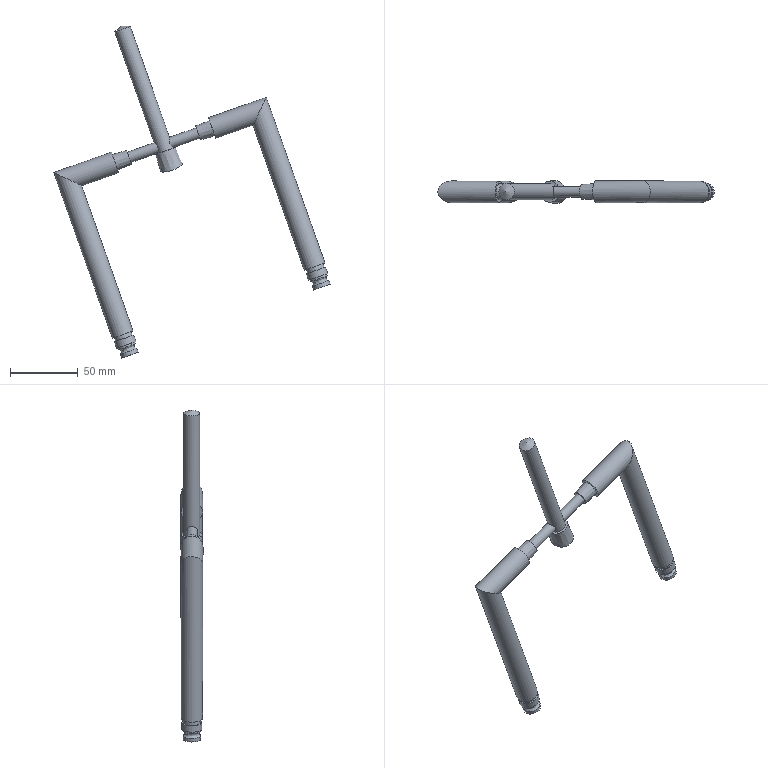Part | STEP file | COOLING-SLIDE1_id166_x_t | 1 solid | 35 faces | box 203.633 x 17.057 x 244.616 mm | volume 86128 mm3 | cylinder 15 | plane 14 | cone 4 | other 2 | commonest cylinder face diameters 13 x6 16 x4 8 x2 15 x2 12 x1
STEP:
#1=CARTESIAN_POINT('',(156.946,0.,-294.272));
#2=VERTEX_POINT('',#1);
#3=CARTESIAN_POINT('',(163.073,0.,-292.102));
#4=DIRECTION('',(-0.3338,0.,0.9426));
#5=DIRECTION('',(-0.9426,0.,-0.3338));
#6=AXIS2_PLACEMENT_3D('',#3,#4,#5);
#7=CIRCLE('',#6,6.5);
#8=EDGE_CURVE('',#2,#2,#7,.T.);
#9=ORIENTED_EDGE('',*,*,#8,.F.);
#10=EDGE_LOOP('',(#9));
#11=FACE_OUTER_BOUND('',#10,.T.);
#12=CARTESIAN_POINT('',(163.073,0.,-292.102));
#13=DIRECTION('',(0.3338,0.,-0.9426));
#14=DIRECTION('',(-0.9426,0.,-0.3338));
#15=AXIS2_PLACEMENT_3D('',#12,#13,#14);
#16=PLANE('',#15);
#17=ADVANCED_FACE('',(#11),#16,.T.);
#18=ORIENTED_EDGE('',*,*,#8,.T.);
#19=EDGE_LOOP('',(#18));
#20=FACE_BOUND('',#19,.T.);
#21=CARTESIAN_POINT('',(168.248,0.,-287.245));
#22=VERTEX_POINT('',#21);
#23=CARTESIAN_POINT('',(162.121,0.,-289.415));
#24=DIRECTION('',(0.3338,0.,-0.9426));
#25=DIRECTION('',(0.9426,0.,0.3338));
#26=AXIS2_PLACEMENT_3D('',#23,#24,#25);
#27=CIRCLE('',#26,6.5);
#28=EDGE_CURVE('',#22,#22,#27,.T.);
#29=ORIENTED_EDGE('',*,*,#28,.T.);
#30=EDGE_LOOP('',(#29));
#31=FACE_BOUND('',#30,.T.);
#32=CARTESIAN_POINT('',(111.159,0.,-145.502));
#33=DIRECTION('',(0.3338,0.,-0.9426));
#34=DIRECTION('',(-0.9426,0.,-0.3338));
#35=AXIS2_PLACEMENT_3D('',#32,#33,#34);
#36=CYLINDRICAL_SURFACE('',#35,6.5);
#37=ADVANCED_FACE('',(#20,#31),#36,.T.);
#38=ORIENTED_EDGE('',*,*,#28,.F.);
#39=EDGE_LOOP('',(#38));
#40=FACE_BOUND('',#39,.T.);
#41=CARTESIAN_POINT('',(154.754,0.,-288.082));
#42=VERTEX_POINT('',#41);
#43=CARTESIAN_POINT('',(160.881,0.,-285.912));
#44=DIRECTION('',(-0.3338,0.,0.9426));
#45=DIRECTION('',(-0.9426,0.,-0.3338));
#46=AXIS2_PLACEMENT_3D('',#43,#44,#45);
#47=CIRCLE('',#46,6.5);
#48=EDGE_CURVE('',#42,#42,#47,.T.);
#49=ORIENTED_EDGE('',*,*,#48,.F.);
#50=EDGE_LOOP('',(#49));
#51=FACE_BOUND('',#50,.T.);
#52=CARTESIAN_POINT('',(168.326,0.,-285.247));
#53=DIRECTION('',(0.,-1.,0.));
#54=DIRECTION('',(0.9426,0.,0.3338));
#55=AXIS2_PLACEMENT_3D('',#52,#53,#54);
#56=CIRCLE('',#55,2.);
#57=CARTESIAN_POINT('',(161.501,0.,-287.664));
#58=DIRECTION('',(0.3338,0.,-0.9426));
#59=AXIS1_PLACEMENT('',#57,#58);
#60=SURFACE_OF_REVOLUTION('',#56,#59);
#61=ADVANCED_FACE('',(#40,#51),#60,.T.);
#62=ORIENTED_EDGE('',*,*,#48,.T.);
#63=EDGE_LOOP('',(#62));
#64=FACE_BOUND('',#63,.T.);
#65=CARTESIAN_POINT('',(154.275,0.,-286.731));
#66=VERTEX_POINT('',#65);
#67=CARTESIAN_POINT('',(160.402,0.,-284.561));
#68=DIRECTION('',(-0.3338,0.,0.9426));
#69=DIRECTION('',(-0.9426,0.,-0.3338));
#70=AXIS2_PLACEMENT_3D('',#67,#68,#69);
#71=CIRCLE('',#70,6.5);
#72=EDGE_CURVE('',#66,#66,#71,.T.);
#73=ORIENTED_EDGE('',*,*,#72,.F.);
#74=EDGE_LOOP('',(#73));
#75=FACE_BOUND('',#74,.T.);
#76=CARTESIAN_POINT('',(111.159,0.,-145.502));
#77=DIRECTION('',(0.3338,0.,-0.9426));
#78=DIRECTION('',(-0.9426,0.,-0.3338));
#79=AXIS2_PLACEMENT_3D('',#76,#77,#78);
#80=CYLINDRICAL_SURFACE('',#79,6.5);
#81=ADVANCED_FACE('',(#64,#75),#80,.T.);
#82=ORIENTED_EDGE('',*,*,#72,.T.);
#83=EDGE_LOOP('',(#82));
#84=FACE_BOUND('',#83,.T.);
#85=CARTESIAN_POINT('',(153.332,0.,-287.065));
#86=VERTEX_POINT('',#85);
#87=CARTESIAN_POINT('',(160.402,0.,-284.561));
#88=DIRECTION('',(-0.3338,0.,0.9426));
#89=DIRECTION('',(-0.9426,0.,-0.3338));
#90=AXIS2_PLACEMENT_3D('',#87,#88,#89);
#91=CIRCLE('',#90,7.5);
#92=EDGE_CURVE('',#86,#86,#91,.T.);
#93=ORIENTED_EDGE('',*,*,#92,.F.);
#94=EDGE_LOOP('',(#93));
#95=FACE_BOUND('',#94,.T.);
#96=CARTESIAN_POINT('',(160.402,0.,-284.561));
#97=DIRECTION('',(0.3338,0.,-0.9426));
#98=DIRECTION('',(-0.9426,0.,-0.3338));
#99=AXIS2_PLACEMENT_3D('',#96,#97,#98);
#100=PLANE('',#99);
#101=ADVANCED_FACE('',(#84,#95),#100,.T.);
#102=CARTESIAN_POINT('',(151.663,0.,-282.351));
#103=VERTEX_POINT('',#102);
#104=CARTESIAN_POINT('',(158.733,0.,-279.848));
#105=DIRECTION('',(0.3338,0.,-0.9426));
#106=DIRECTION('',(-0.9426,0.,-0.3338));
#107=AXIS2_PLACEMENT_3D('',#104,#105,#106);
#108=CIRCLE('',#107,7.5);
#109=EDGE_CURVE('',#103,#103,#108,.T.);
#110=ORIENTED_EDGE('',*,*,#109,.T.);
#111=EDGE_LOOP('',(#110));
#112=FACE_BOUND('',#111,.T.);
#113=ORIENTED_EDGE('',*,*,#92,.T.);
#114=EDGE_LOOP('',(#113));
#115=FACE_BOUND('',#114,.T.);
#116=CARTESIAN_POINT('',(111.159,0.,-145.502));
#117=DIRECTION('',(0.3338,0.,-0.9426));
#118=DIRECTION('',(-0.9426,0.,-0.3338));
#119=AXIS2_PLACEMENT_3D('',#116,#117,#118);
#120=CYLINDRICAL_SURFACE('',#119,7.5);
#121=ADVANCED_FACE('',(#112,#115),#120,.T.);
#122=CARTESIAN_POINT('',(152.606,0.,-282.018));
#123=VERTEX_POINT('',#122);
#124=CARTESIAN_POINT('',(158.733,0.,-279.848));
#125=DIRECTION('',(-0.3338,0.,0.9426));
#126=DIRECTION('',(-0.9426,0.,-0.3338));
#127=AXIS2_PLACEMENT_3D('',#124,#125,#126);
#128=CIRCLE('',#127,6.5);
#129=EDGE_CURVE('',#123,#123,#128,.T.);
#130=ORIENTED_EDGE('',*,*,#129,.F.);
#131=EDGE_LOOP('',(#130));
#132=FACE_BOUND('',#131,.T.);
#133=ORIENTED_EDGE('',*,*,#109,.F.);
#134=EDGE_LOOP('',(#133));
#135=FACE_BOUND('',#134,.T.);
#136=CARTESIAN_POINT('',(158.733,0.,-279.848));
#137=DIRECTION('',(0.3338,0.,-0.9426));
#138=DIRECTION('',(-0.9426,0.,-0.3338));
#139=AXIS2_PLACEMENT_3D('',#136,#137,#138);
#140=PLANE('',#139);
#141=ADVANCED_FACE('',(#132,#135),#140,.F.);
#142=ORIENTED_EDGE('',*,*,#129,.T.);
#143=EDGE_LOOP('',(#142));
#144=FACE_BOUND('',#143,.T.);
#145=CARTESIAN_POINT('',(151.605,0.,-279.19));
#146=VERTEX_POINT('',#145);
#147=CARTESIAN_POINT('',(157.732,0.,-277.02));
#148=DIRECTION('',(-0.3338,0.,0.9426));
#149=DIRECTION('',(-0.9426,0.,-0.3338));
#150=AXIS2_PLACEMENT_3D('',#147,#148,#149);
#151=CIRCLE('',#150,6.5);
#152=EDGE_CURVE('',#146,#146,#151,.T.);
#153=ORIENTED_EDGE('',*,*,#152,.F.);
#154=EDGE_LOOP('',(#153));
#155=FACE_BOUND('',#154,.T.);
#156=CARTESIAN_POINT('',(111.159,0.,-145.502));
#157=DIRECTION('',(0.3338,0.,-0.9426));
#158=DIRECTION('',(-0.9426,0.,-0.3338));
#159=AXIS2_PLACEMENT_3D('',#156,#157,#158);
#160=CYLINDRICAL_SURFACE('',#159,6.5);
#161=ADVANCED_FACE('',(#144,#155),#160,.T.);
#162=ORIENTED_EDGE('',*,*,#152,.T.);
#163=EDGE_LOOP('',(#162));
#164=FACE_BOUND('',#163,.T.);
#165=CARTESIAN_POINT('',(150.191,0.,-279.69));
#166=VERTEX_POINT('',#165);
#167=CARTESIAN_POINT('',(157.732,0.,-277.02));
#168=DIRECTION('',(-0.3338,0.,0.9426));
#169=DIRECTION('',(-0.9426,0.,-0.3338));
#170=AXIS2_PLACEMENT_3D('',#167,#168,#169);
#171=CIRCLE('',#170,8.);
#172=EDGE_CURVE('',#166,#166,#171,.T.);
#173=ORIENTED_EDGE('',*,*,#172,.F.);
#174=EDGE_LOOP('',(#173));
#175=FACE_BOUND('',#174,.T.);
#176=CARTESIAN_POINT('',(157.732,0.,-277.02));
#177=DIRECTION('',(0.3338,0.,-0.9426));
#178=DIRECTION('',(-0.9426,0.,-0.3338));
#179=AXIS2_PLACEMENT_3D('',#176,#177,#178);
#180=PLANE('',#179);
#181=ADVANCED_FACE('',(#164,#175),#180,.T.);
#182=ORIENTED_EDGE('',*,*,#172,.T.);
#183=EDGE_LOOP('',(#182));
#184=FACE_BOUND('',#183,.T.);
#185=CARTESIAN_POINT('',(112.304,0.,-172.701));
#186=VERTEX_POINT('',#185);
#187=CARTESIAN_POINT('',(117.174,0.,-162.489));
#188=DIRECTION('',(-0.9026,0.,0.4305));
#189=DIRECTION('',(-0.4305,0.,-0.9026));
#190=AXIS2_PLACEMENT_3D('',#187,#188,#189);
#191=ELLIPSE('',#190,11.314,8.);
#192=EDGE_CURVE('',#186,#186,#191,.T.);
#193=ORIENTED_EDGE('',*,*,#192,.F.);
#194=EDGE_LOOP('',(#193));
#195=FACE_BOUND('',#194,.T.);
#196=CARTESIAN_POINT('',(111.159,0.,-145.502));
#197=DIRECTION('',(0.3338,0.,-0.9426));
#198=DIRECTION('',(-0.9426,0.,-0.3338));
#199=AXIS2_PLACEMENT_3D('',#196,#197,#198);
#200=CYLINDRICAL_SURFACE('',#199,8.);
#201=ADVANCED_FACE('',(#184,#195),#200,.T.);
#202=CARTESIAN_POINT('',(79.626,0.,-167.299));
#203=VERTEX_POINT('',#202);
#204=CARTESIAN_POINT('',(82.297,0.,-174.84));
#205=DIRECTION('',(-0.9426,0.,-0.3338));
#206=DIRECTION('',(-0.3338,0.,0.9426));
#207=AXIS2_PLACEMENT_3D('',#204,#205,#206);
#208=CIRCLE('',#207,8.);
#209=EDGE_CURVE('',#203,#203,#208,.T.);
#210=ORIENTED_EDGE('',*,*,#209,.F.);
#211=EDGE_LOOP('',(#210));
#212=FACE_BOUND('',#211,.T.);
#213=ORIENTED_EDGE('',*,*,#192,.T.);
#214=EDGE_LOOP('',(#213));
#215=FACE_BOUND('',#214,.T.);
#216=CARTESIAN_POINT('',(135.149,0.,-156.124));
#217=DIRECTION('',(-0.9426,0.,-0.3338));
#218=DIRECTION('',(-0.3338,0.,0.9426));
#219=AXIS2_PLACEMENT_3D('',#216,#217,#218);
#220=CYLINDRICAL_SURFACE('',#219,8.);
#221=ADVANCED_FACE('',(#212,#215),#220,.T.);
#222=CARTESIAN_POINT('',(84.299,0.,-180.496));
#223=VERTEX_POINT('',#222);
#224=CARTESIAN_POINT('',(82.297,0.,-174.84));
#225=DIRECTION('',(-0.9426,0.,-0.3338));
#226=DIRECTION('',(0.3338,0.,-0.9426));
#227=AXIS2_PLACEMENT_3D('',#224,#225,#226);
#228=CIRCLE('',#227,6.);
#229=EDGE_CURVE('',#223,#223,#228,.T.);
#230=ORIENTED_EDGE('',*,*,#229,.F.);
#231=EDGE_LOOP('',(#230));
#232=FACE_BOUND('',#231,.T.);
#233=ORIENTED_EDGE('',*,*,#209,.T.);
#234=EDGE_LOOP('',(#233));
#235=FACE_BOUND('',#234,.T.);
#236=CARTESIAN_POINT('',(82.297,0.,-174.84));
#237=DIRECTION('',(-0.9426,0.,-0.3338));
#238=DIRECTION('',(-0.3338,0.,0.9426));
#239=AXIS2_PLACEMENT_3D('',#236,#237,#238);
#240=PLANE('',#239);
#241=ADVANCED_FACE('',(#232,#235),#240,.T.);
#242=CARTESIAN_POINT('',(15.549,0.,-344.343));
#243=VERTEX_POINT('',#242);
#244=CARTESIAN_POINT('',(21.676,0.,-342.173));
#245=DIRECTION('',(-0.3338,0.,0.9426));
#246=DIRECTION('',(-0.9426,0.,-0.3338));
#247=AXIS2_PLACEMENT_3D('',#244,#245,#246);
#248=CIRCLE('',#247,6.5);
#249=EDGE_CURVE('',#243,#243,#248,.T.);
#250=ORIENTED_EDGE('',*,*,#249,.F.);
#251=EDGE_LOOP('',(#250));
#252=FACE_OUTER_BOUND('',#251,.T.);
#253=CARTESIAN_POINT('',(21.676,0.,-342.173));
#254=DIRECTION('',(0.3338,0.,-0.9426));
#255=DIRECTION('',(-0.9426,0.,-0.3338));
#256=AXIS2_PLACEMENT_3D('',#253,#254,#255);
#257=PLANE('',#256);
#258=ADVANCED_FACE('',(#252),#257,.T.);
#259=CARTESIAN_POINT('',(52.986,-8.659,-205.908));
#260=VERTEX_POINT('',#259);
#261=CARTESIAN_POINT('',(52.276,-0.1301,-203.904));
#262=DIRECTION('',(-0.3239,-0.2419,0.9146));
#263=DIRECTION('',(0.08076,-0.9703,-0.228));
#264=AXIS2_PLACEMENT_3D('',#261,#262,#263);
#265=ELLIPSE('',#264,8.79,8.528);
#266=EDGE_CURVE('',#260,#260,#265,.T.);
#267=ORIENTED_EDGE('',*,*,#266,.F.);
#268=EDGE_LOOP('',(#267));
#269=FACE_OUTER_BOUND('',#268,.T.);
#270=CARTESIAN_POINT('',(110.689,-22.413,-189.112));
#271=DIRECTION('',(-0.3239,-0.2419,0.9146));
#272=DIRECTION('',(0.9426,0.,0.3338));
#273=AXIS2_PLACEMENT_3D('',#270,#271,#272);
#274=PLANE('',#273);
#275=ADVANCED_FACE('',(#269),#274,.F.);
#276=ORIENTED_EDGE('',*,*,#229,.T.);
#277=EDGE_LOOP('',(#276));
#278=FACE_BOUND('',#277,.T.);
#279=CARTESIAN_POINT('',(73.763,0.,-183.696));
#280=VERTEX_POINT('',#279);
#281=CARTESIAN_POINT('',(71.927,0.,-178.512));
#282=DIRECTION('',(-0.9426,0.,-0.3338));
#283=DIRECTION('',(0.3338,0.,-0.9426));
#284=AXIS2_PLACEMENT_3D('',#281,#282,#283);
#285=CIRCLE('',#284,5.5);
#286=EDGE_CURVE('',#280,#280,#285,.T.);
#287=ORIENTED_EDGE('',*,*,#286,.F.);
#288=EDGE_LOOP('',(#287));
#289=FACE_BOUND('',#288,.T.);
#290=CARTESIAN_POINT('',(82.297,0.,-174.84));
#291=DIRECTION('',(0.9426,0.,0.3338));
#292=DIRECTION('',(0.3338,0.,-0.9426));
#293=AXIS2_PLACEMENT_3D('',#290,#291,#292);
#294=CONICAL_SURFACE('',#293,6.,2.603);
#295=ADVANCED_FACE('',(#278,#289),#294,.T.);
#296=ORIENTED_EDGE('',*,*,#249,.T.);
#297=EDGE_LOOP('',(#296));
#298=FACE_BOUND('',#297,.T.);
#299=CARTESIAN_POINT('',(26.852,0.,-337.316));
#300=VERTEX_POINT('',#299);
#301=CARTESIAN_POINT('',(20.725,0.,-339.486));
#302=DIRECTION('',(0.3338,0.,-0.9426));
#303=DIRECTION('',(0.9426,0.,0.3338));
#304=AXIS2_PLACEMENT_3D('',#301,#302,#303);
#305=CIRCLE('',#304,6.5);
#306=EDGE_CURVE('',#300,#300,#305,.T.);
#307=ORIENTED_EDGE('',*,*,#306,.T.);
#308=EDGE_LOOP('',(#307));
#309=FACE_BOUND('',#308,.T.);
#310=CARTESIAN_POINT('',(-30.237,0.,-195.573));
#311=DIRECTION('',(0.3338,0.,-0.9426));
#312=DIRECTION('',(-0.9426,0.,-0.3338));
#313=AXIS2_PLACEMENT_3D('',#310,#311,#312);
#314=CYLINDRICAL_SURFACE('',#313,6.5);
#315=ADVANCED_FACE('',(#298,#309),#314,.T.);
#316=CARTESIAN_POINT('',(40.681,0.,-194.351));
#317=VERTEX_POINT('',#316);
#318=CARTESIAN_POINT('',(47.978,0.,-191.766));
#319=DIRECTION('',(0.3338,0.,-0.9426));
#320=DIRECTION('',(-0.9426,0.,-0.3338));
#321=AXIS2_PLACEMENT_3D('',#318,#319,#320);
#322=CIRCLE('',#321,7.741);
#323=EDGE_CURVE('',#317,#317,#322,.T.);
#324=ORIENTED_EDGE('',*,*,#323,.T.);
#325=EDGE_LOOP('',(#324));
#326=FACE_BOUND('',#325,.T.);
#327=ORIENTED_EDGE('',*,*,#266,.T.);
#328=EDGE_LOOP('',(#327));
#329=FACE_BOUND('',#328,.T.);
#330=CARTESIAN_POINT('',(52.291,0.,-203.946));
#331=DIRECTION('',(0.3338,0.,-0.9426));
#332=DIRECTION('',(-0.9426,0.,-0.3338));
#333=AXIS2_PLACEMENT_3D('',#330,#331,#332);
#334=CONICAL_SURFACE('',#333,8.531,3.5);
#335=ADVANCED_FACE('',(#326,#329),#334,.T.);
#336=CARTESIAN_POINT('',(70.592,0.,-174.741));
#337=VERTEX_POINT('',#336);
#338=CARTESIAN_POINT('',(71.927,0.,-178.512));
#339=DIRECTION('',(-0.9426,0.,-0.3338));
#340=DIRECTION('',(-0.3338,0.,0.9426));
#341=AXIS2_PLACEMENT_3D('',#338,#339,#340);
#342=CIRCLE('',#341,4.);
#343=EDGE_CURVE('',#337,#337,#342,.T.);
#344=ORIENTED_EDGE('',*,*,#343,.F.);
#345=EDGE_LOOP('',(#344));
#346=FACE_BOUND('',#345,.T.);
#347=ORIENTED_EDGE('',*,*,#286,.T.);
#348=EDGE_LOOP('',(#347));
#349=FACE_BOUND('',#348,.T.);
#350=CARTESIAN_POINT('',(71.927,0.,-178.512));
#351=DIRECTION('',(-0.9426,0.,-0.3338));
#352=DIRECTION('',(-0.3338,0.,0.9426));
#353=AXIS2_PLACEMENT_3D('',#350,#351,#352);
#354=PLANE('',#353);
#355=ADVANCED_FACE('',(#346,#349),#354,.T.);
#356=ORIENTED_EDGE('',*,*,#306,.F.);
#357=EDGE_LOOP('',(#356));
#358=FACE_BOUND('',#357,.T.);
#359=CARTESIAN_POINT('',(13.357,0.,-338.153));
#360=VERTEX_POINT('',#359);
#361=CARTESIAN_POINT('',(19.484,0.,-335.983));
#362=DIRECTION('',(-0.3338,0.,0.9426));
#363=DIRECTION('',(-0.9426,0.,-0.3338));
#364=AXIS2_PLACEMENT_3D('',#361,#362,#363);
#365=CIRCLE('',#364,6.5);
#366=EDGE_CURVE('',#360,#360,#365,.T.);
#367=ORIENTED_EDGE('',*,*,#366,.F.);
#368=EDGE_LOOP('',(#367));
#369=FACE_BOUND('',#368,.T.);
#370=CARTESIAN_POINT('',(26.93,0.,-335.318));
#371=DIRECTION('',(0.,-1.,0.));
#372=DIRECTION('',(0.9426,0.,0.3338));
#373=AXIS2_PLACEMENT_3D('',#370,#371,#372);
#374=CIRCLE('',#373,2.);
#375=CARTESIAN_POINT('',(20.105,0.,-337.735));
#376=DIRECTION('',(0.3338,0.,-0.9426));
#377=AXIS1_PLACEMENT('',#375,#376);
#378=SURFACE_OF_REVOLUTION('',#374,#377);
#379=ADVANCED_FACE('',(#358,#369),#378,.T.);
#380=CARTESIAN_POINT('',(10.583,0.,-104.139));
#381=VERTEX_POINT('',#380);
#382=CARTESIAN_POINT('',(16.239,0.,-102.136));
#383=DIRECTION('',(0.3338,0.,-0.9426));
#384=DIRECTION('',(-0.9426,0.,-0.3338));
#385=AXIS2_PLACEMENT_3D('',#382,#383,#384);
#386=CIRCLE('',#385,6.);
#387=EDGE_CURVE('',#381,#381,#386,.T.);
#388=ORIENTED_EDGE('',*,*,#387,.F.);
#389=EDGE_LOOP('',(#388));
#390=FACE_BOUND('',#389,.T.);
#391=CARTESIAN_POINT('',(15.385,0.,-99.727));
#392=VERTEX_POINT('',#391);
#393=VERTEX_LOOP('',#392);
#394=FACE_BOUND('',#393,.T.);
#395=CARTESIAN_POINT('',(16.239,0.,-102.136));
#396=DIRECTION('',(0.3338,0.,-0.9426));
#397=DIRECTION('',(-0.9426,0.,-0.3338));
#398=AXIS2_PLACEMENT_3D('',#395,#396,#397);
#399=CONICAL_SURFACE('',#398,6.,66.921);
#400=ADVANCED_FACE('',(#390,#394),#399,.T.);
#401=CARTESIAN_POINT('',(42.322,0.,-193.769));
#402=VERTEX_POINT('',#401);
#403=CARTESIAN_POINT('',(47.978,0.,-191.766));
#404=DIRECTION('',(-0.3338,0.,0.9426));
#405=DIRECTION('',(-0.9426,0.,-0.3338));
#406=AXIS2_PLACEMENT_3D('',#403,#404,#405);
#407=CIRCLE('',#406,6.);
#408=EDGE_CURVE('',#402,#402,#407,.T.);
#409=ORIENTED_EDGE('',*,*,#408,.F.);
#410=EDGE_LOOP('',(#409));
#411=FACE_BOUND('',#410,.T.);
#412=ORIENTED_EDGE('',*,*,#323,.F.);
#413=EDGE_LOOP('',(#412));
#414=FACE_BOUND('',#413,.T.);
#415=CARTESIAN_POINT('',(47.978,0.,-191.766));
#416=DIRECTION('',(0.3338,0.,-0.9426));
#417=DIRECTION('',(-0.9426,0.,-0.3338));
#418=AXIS2_PLACEMENT_3D('',#415,#416,#417);
#419=PLANE('',#418);
#420=ADVANCED_FACE('',(#411,#414),#419,.F.);
#421=ORIENTED_EDGE('',*,*,#343,.T.);
#422=EDGE_LOOP('',(#421));
#423=FACE_BOUND('',#422,.T.);
#424=CARTESIAN_POINT('',(53.467,0.,-189.292));
#425=VERTEX_POINT('',#424);
#426=CARTESIAN_POINT('',(53.467,1.093,-189.292));
#427=CARTESIAN_POINT('',(53.467,-1.093,-189.292));
#428=CARTESIAN_POINT('',(53.003,-2.12,-188.968));
#429=CARTESIAN_POINT('',(51.805,-3.546,-187.874));
#430=CARTESIAN_POINT('',(51.06,-3.997,-187.064));
#431=CARTESIAN_POINT('',(50.331,-4.003,-185.021));
#432=CARTESIAN_POINT('',(50.396,-3.559,-183.92));
#433=CARTESIAN_POINT('',(50.639,-2.129,-182.299));
#434=CARTESIAN_POINT('',(50.796,-1.105,-181.755));
#435=CARTESIAN_POINT('',(50.798,1.084,-181.748));
#436=CARTESIAN_POINT('',(50.641,2.115,-182.291));
#437=CARTESIAN_POINT('',(50.398,3.545,-183.896));
#438=CARTESIAN_POINT('',(50.328,3.997,-184.996));
#439=CARTESIAN_POINT('',(51.048,4.003,-187.046));
#440=CARTESIAN_POINT('',(51.793,3.558,-187.862));
#441=CARTESIAN_POINT('',(53.003,2.123,-188.968));
#442=CARTESIAN_POINT('',(53.467,1.093,-189.292));
#443=CARTESIAN_POINT('',(53.467,-1.093,-189.292));
#444=B_SPLINE_CURVE_WITH_KNOTS('',3,(#426,#427,#428,#429,#430,#431,#432,#433,#434,#435,#436,#437,#438,#439,#440,#441,#442,#443),.UNSPECIFIED.,.T.,.F.,(2,2,2,2,2,2,2,2,2,2,2),(-0.125,0.,0.125,0.25,0.375,0.5,0.625,0.75,0.875,1.,1.125),.UNSPECIFIED.);
#445=EDGE_CURVE('',#425,#425,#444,.T.);
#446=ORIENTED_EDGE('',*,*,#445,.F.);
#447=EDGE_LOOP('',(#446));
#448=FACE_BOUND('',#447,.T.);
#449=CARTESIAN_POINT('',(135.149,0.,-156.124));
#450=DIRECTION('',(-0.9426,0.,-0.3338));
#451=DIRECTION('',(-0.3338,0.,0.9426));
#452=AXIS2_PLACEMENT_3D('',#449,#450,#451);
#453=CYLINDRICAL_SURFACE('',#452,4.);
#454=ADVANCED_FACE('',(#423,#448),#453,.T.);
#455=ORIENTED_EDGE('',*,*,#366,.T.);
#456=EDGE_LOOP('',(#455));
#457=FACE_BOUND('',#456,.T.);
#458=CARTESIAN_POINT('',(12.879,0.,-336.802));
#459=VERTEX_POINT('',#458);
#460=CARTESIAN_POINT('',(19.006,0.,-334.632));
#461=DIRECTION('',(-0.3338,0.,0.9426));
#462=DIRECTION('',(-0.9426,0.,-0.3338));
#463=AXIS2_PLACEMENT_3D('',#460,#461,#462);
#464=CIRCLE('',#463,6.5);
#465=EDGE_CURVE('',#459,#459,#464,.T.);
#466=ORIENTED_EDGE('',*,*,#465,.F.);
#467=EDGE_LOOP('',(#466));
#468=FACE_BOUND('',#467,.T.);
#469=CARTESIAN_POINT('',(-30.237,0.,-195.573));
#470=DIRECTION('',(0.3338,0.,-0.9426));
#471=DIRECTION('',(-0.9426,0.,-0.3338));
#472=AXIS2_PLACEMENT_3D('',#469,#470,#471);
#473=CYLINDRICAL_SURFACE('',#472,6.5);
#474=ADVANCED_FACE('',(#457,#468),#473,.T.);
#475=ORIENTED_EDGE('',*,*,#387,.T.);
#476=EDGE_LOOP('',(#475));
#477=FACE_BOUND('',#476,.T.);
#478=CARTESIAN_POINT('',(42.156,0.,-193.298));
#479=VERTEX_POINT('',#478);
#480=CARTESIAN_POINT('',(42.156,1.093,-193.298));
#481=CARTESIAN_POINT('',(42.156,-1.093,-193.298));
#482=CARTESIAN_POINT('',(42.312,-2.12,-192.754));
#483=CARTESIAN_POINT('',(42.554,-3.546,-191.15));
#484=CARTESIAN_POINT('',(42.624,-3.997,-190.051));
#485=CARTESIAN_POINT('',(41.905,-4.003,-188.005));
#486=CARTESIAN_POINT('',(41.161,-3.559,-187.19));
#487=CARTESIAN_POINT('',(39.953,-2.129,-186.084));
#488=CARTESIAN_POINT('',(39.488,-1.105,-185.759));
#489=CARTESIAN_POINT('',(39.482,1.084,-185.755));
#490=CARTESIAN_POINT('',(39.946,2.115,-186.079));
#491=CARTESIAN_POINT('',(41.145,3.545,-187.173));
#492=CARTESIAN_POINT('',(41.891,3.997,-187.984));
#493=CARTESIAN_POINT('',(42.622,4.003,-190.03));
#494=CARTESIAN_POINT('',(42.556,3.558,-191.133));
#495=CARTESIAN_POINT('',(42.312,2.123,-192.754));
#496=CARTESIAN_POINT('',(42.156,1.093,-193.298));
#497=CARTESIAN_POINT('',(42.156,-1.093,-193.298));
#498=B_SPLINE_CURVE_WITH_KNOTS('',3,(#480,#481,#482,#483,#484,#485,#486,#487,#488,#489,#490,#491,#492,#493,#494,#495,#496,#497),.UNSPECIFIED.,.T.,.F.,(2,2,2,2,2,2,2,2,2,2,2),(-0.125,0.,0.125,0.25,0.375,0.5,0.625,0.75,0.875,1.,1.125),.UNSPECIFIED.);
#499=EDGE_CURVE('',#479,#479,#498,.T.);
#500=ORIENTED_EDGE('',*,*,#499,.F.);
#501=EDGE_LOOP('',(#500));
#502=FACE_BOUND('',#501,.T.);
#503=ORIENTED_EDGE('',*,*,#408,.T.);
#504=EDGE_LOOP('',(#503));
#505=FACE_BOUND('',#504,.T.);
#506=ORIENTED_EDGE('',*,*,#445,.T.);
#507=EDGE_LOOP('',(#506));
#508=FACE_BOUND('',#507,.T.);
#509=CARTESIAN_POINT('',(13.353,0.,-93.987));
#510=DIRECTION('',(0.3338,0.,-0.9426));
#511=DIRECTION('',(-0.9426,0.,-0.3338));
#512=AXIS2_PLACEMENT_3D('',#509,#510,#511);
#513=CYLINDRICAL_SURFACE('',#512,6.);
#514=ADVANCED_FACE('',(#477,#502,#505,#508),#513,.T.);
#515=ORIENTED_EDGE('',*,*,#465,.T.);
#516=EDGE_LOOP('',(#515));
#517=FACE_BOUND('',#516,.T.);
#518=CARTESIAN_POINT('',(11.936,0.,-337.136));
#519=VERTEX_POINT('',#518);
#520=CARTESIAN_POINT('',(19.006,0.,-334.632));
#521=DIRECTION('',(-0.3338,0.,0.9426));
#522=DIRECTION('',(-0.9426,0.,-0.3338));
#523=AXIS2_PLACEMENT_3D('',#520,#521,#522);
#524=CIRCLE('',#523,7.5);
#525=EDGE_CURVE('',#519,#519,#524,.T.);
#526=ORIENTED_EDGE('',*,*,#525,.F.);
#527=EDGE_LOOP('',(#526));
#528=FACE_BOUND('',#527,.T.);
#529=CARTESIAN_POINT('',(19.006,0.,-334.632));
#530=DIRECTION('',(0.3338,0.,-0.9426));
#531=DIRECTION('',(-0.9426,0.,-0.3338));
#532=AXIS2_PLACEMENT_3D('',#529,#530,#531);
#533=PLANE('',#532);
#534=ADVANCED_FACE('',(#517,#528),#533,.T.);
#535=CARTESIAN_POINT('',(19.69,0.,-192.767));
#536=VERTEX_POINT('',#535);
#537=CARTESIAN_POINT('',(21.025,0.,-196.537));
#538=DIRECTION('',(0.9426,0.,0.3338));
#539=DIRECTION('',(-0.3338,0.,0.9426));
#540=AXIS2_PLACEMENT_3D('',#537,#538,#539);
#541=CIRCLE('',#540,4.);
#542=EDGE_CURVE('',#536,#536,#541,.T.);
#543=ORIENTED_EDGE('',*,*,#542,.T.);
#544=EDGE_LOOP('',(#543));
#545=FACE_BOUND('',#544,.T.);
#546=ORIENTED_EDGE('',*,*,#499,.T.);
#547=EDGE_LOOP('',(#546));
#548=FACE_BOUND('',#547,.T.);
#549=CARTESIAN_POINT('',(135.149,0.,-156.124));
#550=DIRECTION('',(-0.9426,0.,-0.3338));
#551=DIRECTION('',(-0.3338,0.,0.9426));
#552=AXIS2_PLACEMENT_3D('',#549,#550,#551);
#553=CYLINDRICAL_SURFACE('',#552,4.);
#554=ADVANCED_FACE('',(#545,#548),#553,.T.);
#555=CARTESIAN_POINT('',(10.267,0.,-332.422));
#556=VERTEX_POINT('',#555);
#557=CARTESIAN_POINT('',(17.337,0.,-329.919));
#558=DIRECTION('',(0.3338,0.,-0.9426));
#559=DIRECTION('',(-0.9426,0.,-0.3338));
#560=AXIS2_PLACEMENT_3D('',#557,#558,#559);
#561=CIRCLE('',#560,7.5);
#562=EDGE_CURVE('',#556,#556,#561,.T.);
#563=ORIENTED_EDGE('',*,*,#562,.T.);
#564=EDGE_LOOP('',(#563));
#565=FACE_BOUND('',#564,.T.);
#566=ORIENTED_EDGE('',*,*,#525,.T.);
#567=EDGE_LOOP('',(#566));
#568=FACE_BOUND('',#567,.T.);
#569=CARTESIAN_POINT('',(-30.237,0.,-195.573));
#570=DIRECTION('',(0.3338,0.,-0.9426));
#571=DIRECTION('',(-0.9426,0.,-0.3338));
#572=AXIS2_PLACEMENT_3D('',#569,#570,#571);
#573=CYLINDRICAL_SURFACE('',#572,7.5);
#574=ADVANCED_FACE('',(#565,#568),#573,.T.);
#575=ORIENTED_EDGE('',*,*,#542,.F.);
#576=EDGE_LOOP('',(#575));
#577=FACE_BOUND('',#576,.T.);
#578=CARTESIAN_POINT('',(19.189,0.,-191.353));
#579=VERTEX_POINT('',#578);
#580=CARTESIAN_POINT('',(21.025,0.,-196.537));
#581=DIRECTION('',(-0.9426,0.,-0.3338));
#582=DIRECTION('',(-0.3338,0.,0.9426));
#583=AXIS2_PLACEMENT_3D('',#580,#581,#582);
#584=CIRCLE('',#583,5.5);
#585=EDGE_CURVE('',#579,#579,#584,.T.);
#586=ORIENTED_EDGE('',*,*,#585,.F.);
#587=EDGE_LOOP('',(#586));
#588=FACE_BOUND('',#587,.T.);
#589=CARTESIAN_POINT('',(21.025,0.,-196.537));
#590=DIRECTION('',(-0.9426,0.,-0.3338));
#591=DIRECTION('',(-0.3338,0.,0.9426));
#592=AXIS2_PLACEMENT_3D('',#589,#590,#591);
#593=PLANE('',#592);
#594=ADVANCED_FACE('',(#577,#588),#593,.F.);
#595=CARTESIAN_POINT('',(11.21,0.,-332.089));
#596=VERTEX_POINT('',#595);
#597=CARTESIAN_POINT('',(17.337,0.,-329.919));
#598=DIRECTION('',(-0.3338,0.,0.9426));
#599=DIRECTION('',(-0.9426,0.,-0.3338));
#600=AXIS2_PLACEMENT_3D('',#597,#598,#599);
#601=CIRCLE('',#600,6.5);
#602=EDGE_CURVE('',#596,#596,#601,.T.);
#603=ORIENTED_EDGE('',*,*,#602,.F.);
#604=EDGE_LOOP('',(#603));
#605=FACE_BOUND('',#604,.T.);
#606=ORIENTED_EDGE('',*,*,#562,.F.);
#607=EDGE_LOOP('',(#606));
#608=FACE_BOUND('',#607,.T.);
#609=CARTESIAN_POINT('',(17.337,0.,-329.919));
#610=DIRECTION('',(0.3338,0.,-0.9426));
#611=DIRECTION('',(-0.9426,0.,-0.3338));
#612=AXIS2_PLACEMENT_3D('',#609,#610,#611);
#613=PLANE('',#612);
#614=ADVANCED_FACE('',(#605,#608),#613,.F.);
#615=CARTESIAN_POINT('',(8.653,0.,-194.553));
#616=VERTEX_POINT('',#615);
#617=CARTESIAN_POINT('',(10.656,0.,-200.209));
#618=DIRECTION('',(0.9426,0.,0.3338));
#619=DIRECTION('',(-0.3338,0.,0.9426));
#620=AXIS2_PLACEMENT_3D('',#617,#618,#619);
#621=CIRCLE('',#620,6.);
#622=EDGE_CURVE('',#616,#616,#621,.T.);
#623=ORIENTED_EDGE('',*,*,#622,.T.);
#624=EDGE_LOOP('',(#623));
#625=FACE_BOUND('',#624,.T.);
#626=ORIENTED_EDGE('',*,*,#585,.T.);
#627=EDGE_LOOP('',(#626));
#628=FACE_BOUND('',#627,.T.);
#629=CARTESIAN_POINT('',(10.656,0.,-200.209));
#630=DIRECTION('',(-0.9426,0.,-0.3338));
#631=DIRECTION('',(-0.3338,0.,0.9426));
#632=AXIS2_PLACEMENT_3D('',#629,#630,#631);
#633=CONICAL_SURFACE('',#632,6.,2.603);
#634=ADVANCED_FACE('',(#625,#628),#633,.T.);
#635=ORIENTED_EDGE('',*,*,#602,.T.);
#636=EDGE_LOOP('',(#635));
#637=FACE_BOUND('',#636,.T.);
#638=CARTESIAN_POINT('',(10.208,0.,-329.261));
#639=VERTEX_POINT('',#638);
#640=CARTESIAN_POINT('',(16.336,0.,-327.091));
#641=DIRECTION('',(-0.3338,0.,0.9426));
#642=DIRECTION('',(-0.9426,0.,-0.3338));
#643=AXIS2_PLACEMENT_3D('',#640,#641,#642);
#644=CIRCLE('',#643,6.5);
#645=EDGE_CURVE('',#639,#639,#644,.T.);
#646=ORIENTED_EDGE('',*,*,#645,.F.);
#647=EDGE_LOOP('',(#646));
#648=FACE_BOUND('',#647,.T.);
#649=CARTESIAN_POINT('',(-30.237,0.,-195.573));
#650=DIRECTION('',(0.3338,0.,-0.9426));
#651=DIRECTION('',(-0.9426,0.,-0.3338));
#652=AXIS2_PLACEMENT_3D('',#649,#650,#651);
#653=CYLINDRICAL_SURFACE('',#652,6.5);
#654=ADVANCED_FACE('',(#637,#648),#653,.T.);
#655=ORIENTED_EDGE('',*,*,#622,.F.);
#656=EDGE_LOOP('',(#655));
#657=FACE_BOUND('',#656,.T.);
#658=CARTESIAN_POINT('',(7.985,0.,-192.668));
#659=VERTEX_POINT('',#658);
#660=CARTESIAN_POINT('',(10.656,0.,-200.209));
#661=DIRECTION('',(-0.9426,0.,-0.3338));
#662=DIRECTION('',(-0.3338,0.,0.9426));
#663=AXIS2_PLACEMENT_3D('',#660,#661,#662);
#664=CIRCLE('',#663,8.);
#665=EDGE_CURVE('',#659,#659,#664,.T.);
#666=ORIENTED_EDGE('',*,*,#665,.F.);
#667=EDGE_LOOP('',(#666));
#668=FACE_BOUND('',#667,.T.);
#669=CARTESIAN_POINT('',(10.656,0.,-200.209));
#670=DIRECTION('',(-0.9426,0.,-0.3338));
#671=DIRECTION('',(-0.3338,0.,0.9426));
#672=AXIS2_PLACEMENT_3D('',#669,#670,#671);
#673=PLANE('',#672);
#674=ADVANCED_FACE('',(#657,#668),#673,.F.);
#675=ORIENTED_EDGE('',*,*,#645,.T.);
#676=EDGE_LOOP('',(#675));
#677=FACE_BOUND('',#676,.T.);
#678=CARTESIAN_POINT('',(8.794,0.,-329.761));
#679=VERTEX_POINT('',#678);
#680=CARTESIAN_POINT('',(16.336,0.,-327.091));
#681=DIRECTION('',(-0.3338,0.,0.9426));
#682=DIRECTION('',(-0.9426,0.,-0.3338));
#683=AXIS2_PLACEMENT_3D('',#680,#681,#682);
#684=CIRCLE('',#683,8.);
#685=EDGE_CURVE('',#679,#679,#684,.T.);
#686=ORIENTED_EDGE('',*,*,#685,.F.);
#687=EDGE_LOOP('',(#686));
#688=FACE_BOUND('',#687,.T.);
#689=CARTESIAN_POINT('',(16.336,0.,-327.091));
#690=DIRECTION('',(0.3338,0.,-0.9426));
#691=DIRECTION('',(-0.9426,0.,-0.3338));
#692=AXIS2_PLACEMENT_3D('',#689,#690,#691);
#693=PLANE('',#692);
#694=ADVANCED_FACE('',(#677,#688),#693,.T.);
#695=ORIENTED_EDGE('',*,*,#665,.T.);
#696=EDGE_LOOP('',(#695));
#697=FACE_BOUND('',#696,.T.);
#698=CARTESIAN_POINT('',(-14.01,0.,-217.431));
#699=VERTEX_POINT('',#698);
#700=CARTESIAN_POINT('',(-24.222,0.,-212.56));
#701=DIRECTION('',(-0.4305,0.,-0.9026));
#702=DIRECTION('',(0.9026,0.,-0.4305));
#703=AXIS2_PLACEMENT_3D('',#700,#701,#702);
#704=ELLIPSE('',#703,11.314,8.);
#705=EDGE_CURVE('',#699,#699,#704,.T.);
#706=ORIENTED_EDGE('',*,*,#705,.F.);
#707=EDGE_LOOP('',(#706));
#708=FACE_BOUND('',#707,.T.);
#709=CARTESIAN_POINT('',(135.149,0.,-156.124));
#710=DIRECTION('',(-0.9426,0.,-0.3338));
#711=DIRECTION('',(-0.3338,0.,0.9426));
#712=AXIS2_PLACEMENT_3D('',#709,#710,#711);
#713=CYLINDRICAL_SURFACE('',#712,8.);
#714=ADVANCED_FACE('',(#697,#708),#713,.T.);
#715=ORIENTED_EDGE('',*,*,#685,.T.);
#716=EDGE_LOOP('',(#715));
#717=FACE_BOUND('',#716,.T.);
#718=ORIENTED_EDGE('',*,*,#705,.T.);
#719=EDGE_LOOP('',(#718));
#720=FACE_BOUND('',#719,.T.);
#721=CARTESIAN_POINT('',(-30.237,0.,-195.573));
#722=DIRECTION('',(0.3338,0.,-0.9426));
#723=DIRECTION('',(-0.9426,0.,-0.3338));
#724=AXIS2_PLACEMENT_3D('',#721,#722,#723);
#725=CYLINDRICAL_SURFACE('',#724,8.);
#726=ADVANCED_FACE('',(#717,#720),#725,.T.);
#727=CLOSED_SHELL('',(#17,#37,#61,#81,#101,#121,#141,#161,#181,#201,#221,#241,#258,#275,#295,#315,#335,#355,#379,#400,#420,#454,#474,#514,#534,#554,#574,#594,#614,#634,#654,#674,#694,#714,#726));
#728=MANIFOLD_SOLID_BREP('',#727);
#729=(LENGTH_UNIT()NAMED_UNIT(*)SI_UNIT(.MILLI.,.METRE.));
#730=UNCERTAINTY_MEASURE_WITH_UNIT(LENGTH_MEASURE(0.0508),#729,'','');
#731=(NAMED_UNIT(*)PLANE_ANGLE_UNIT()SI_UNIT($,.RADIAN.));
#732=PLANE_ANGLE_MEASURE_WITH_UNIT(PLANE_ANGLE_MEASURE(0.01745),#731);
#733=DIMENSIONAL_EXPONENTS(0.,0.,0.,0.,0.,0.,0.);
#734=(CONVERSION_BASED_UNIT('DEGREE',#732)NAMED_UNIT(#733)PLANE_ANGLE_UNIT());
#735=(NAMED_UNIT(*)SI_UNIT($,.STERADIAN.)SOLID_ANGLE_UNIT());
#736=(GEOMETRIC_REPRESENTATION_CONTEXT(3)GLOBAL_UNCERTAINTY_ASSIGNED_CONTEXT((#730))GLOBAL_UNIT_ASSIGNED_CONTEXT((#729,#734,#735))REPRESENTATION_CONTEXT('',''));
#737=ADVANCED_BREP_SHAPE_REPRESENTATION('',(#728),#736);